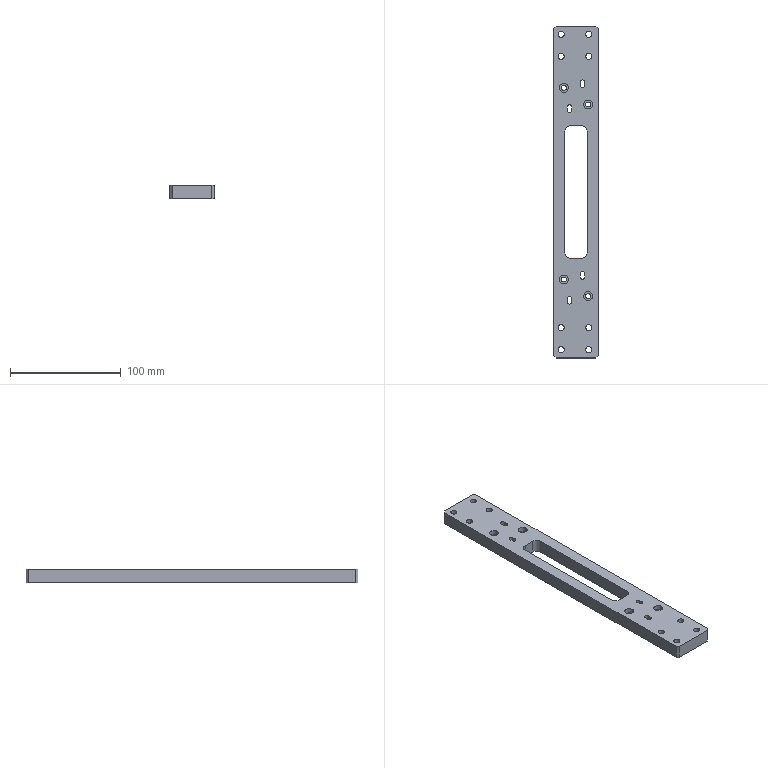Part | SolidWorks | features Cut 3, Chamfer 2, HoleWzd 2, ICE 2, Extrusion 1, Fillet 1 | 1 solid | 94 faces | box 40 x 300 x 12 mm | volume 108008 mm3 | cylinder 60 | plane 34 | commonest cylinder face diameters 10 x20 5.5 x16 4 x8 4.5 x8 8 x8